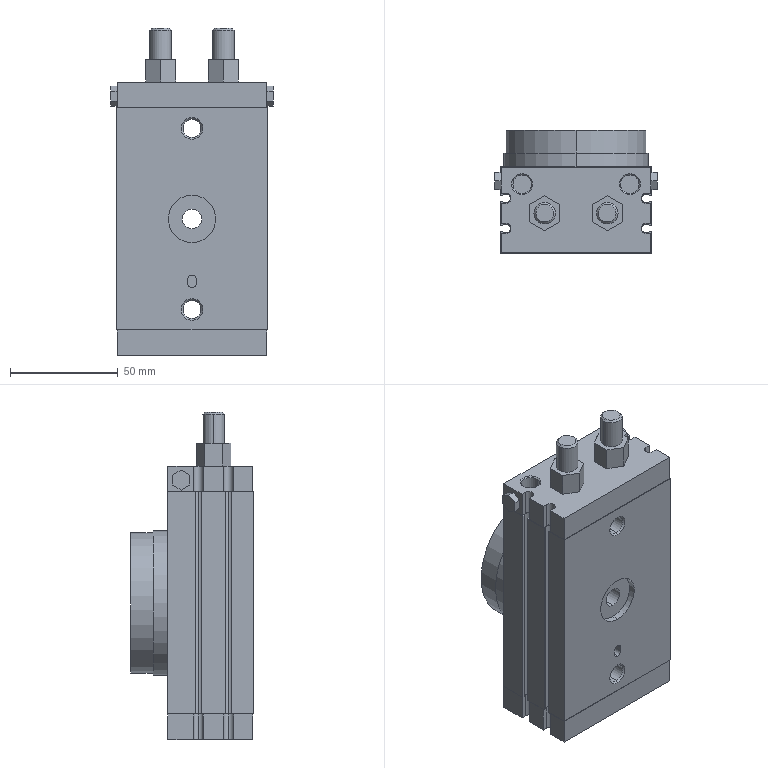Part | STEP file | Revolve气缸-2 | 1 solid | 234 faces | box 75.4 x 57 x 152 mm | volume 392016 mm3 | plane 109 | cylinder 81 | cone 44 | commonest cylinder face diameters 4.917 x24 4.6 x12 4 x9 4.2 x6 8.376 x4 8.566 x4